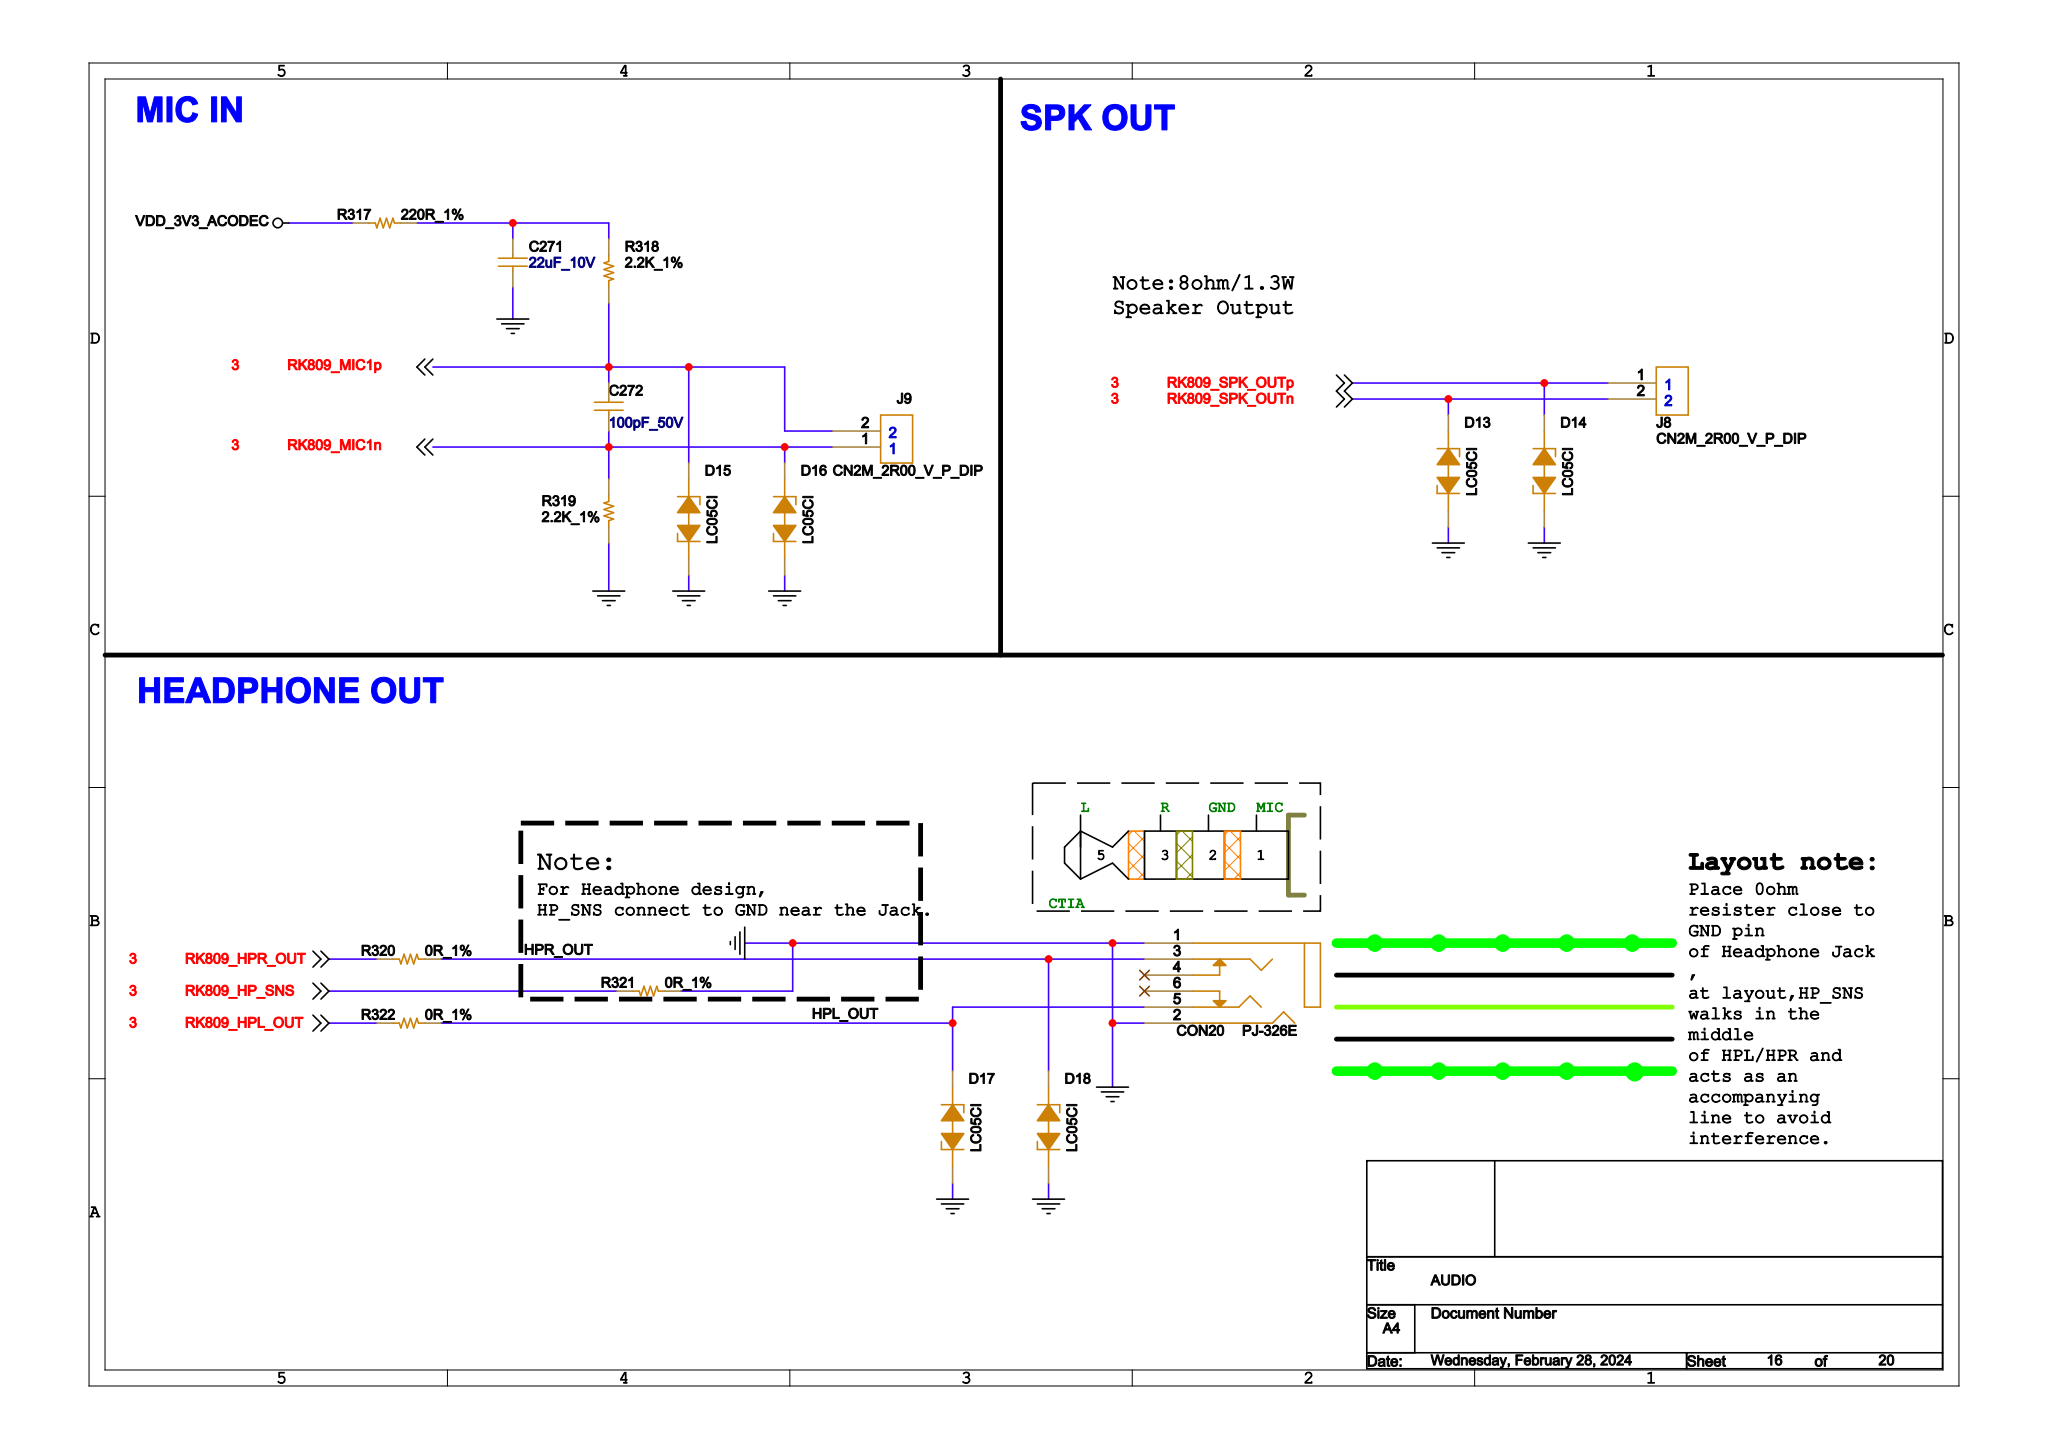Circuit board | Cadence Allegro | 1024 parts | 682 nets | one sheet of the schematic
Parts on this sheet (reference | value | footprint):
C271 | 22uF_10V | C0603
C272 | 100pF_50V | C0603
CON20 | JQ-PJ-3106A-1 | PJ-342E
J8 | CN2M_2R00_V_P_DIP | CN2M_2R00_V_P_DIP
J9 | CN2M_2R00_V_P_DIP | CN2M_2R00_V_P_DIP
R317 | 220R_1% | R0603
R318 | 2.2K_1% | R0603
R319 | 2.2K_1% | R0603
R320 | 0R_1% | R0402
R321 | 0R_1% | R0402
R322 | 0R_1% | R0402
Nets of these parts (net: part-pin ...):
GND: C271-2 CON20-1 CON20-2 R319-2 R321-2
VDD_3V3_ACODEC: R317-1
RK809_HP_SNS: R321-1
RK809_HPL_OUT: R322-1
RK809_HPR_OUT: R320-1
N21590078: C271-1 R317-2 R318-1
RK809_SPK_OUTP: J8-1
RK809_SPK_OUTN: J8-2
RK809_MIC1P: C272-1 J9-2 R318-2
RK809_MIC1N: C272-2 J9-1 R319-1
HPR_OUT: CON20-3 R320-2
HPL_OUT: CON20-5 R322-2